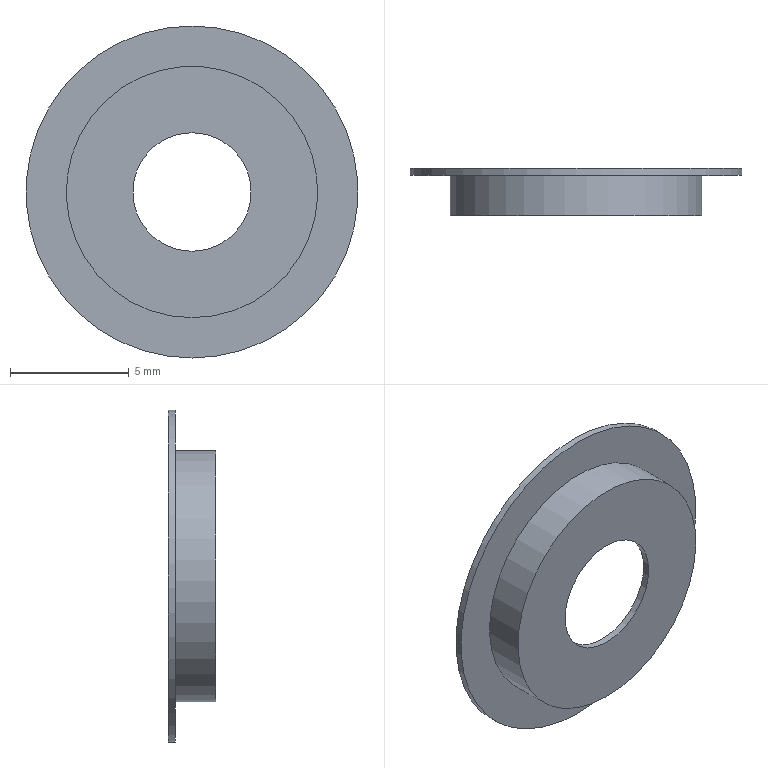Part | NX | features DATUM_CSYS 3, SKETCH 2, SWP104 1 | 1 solid | 8 faces | box 14 x 2 x 14 mm | volume 56.794 mm3 | cylinder 4 | plane 4 | commonest cylinder face diameters 5 x1 10 x1 10.6 x1 14 x1
STEP:
#1=CARTESIAN_POINT('',(0.,0.,-5.));
#2=VERTEX_POINT('',#1);
#3=CARTESIAN_POINT('',(0.,0.,0.));
#4=DIRECTION('',(0.,-1.,0.));
#5=DIRECTION('',(0.,0.,-1.));
#6=AXIS2_PLACEMENT_3D('',#3,#4,#5);
#7=CIRCLE('',#6,5.);
#8=EDGE_CURVE('',#2,#2,#7,.T.);
#9=ORIENTED_EDGE('',*,*,#8,.T.);
#10=EDGE_LOOP('',(#9));
#11=FACE_BOUND('',#10,.T.);
#12=CARTESIAN_POINT('',(0.,1.7,-5.));
#13=VERTEX_POINT('',#12);
#14=CARTESIAN_POINT('',(0.,1.7,0.));
#15=DIRECTION('',(0.,-1.,0.));
#16=DIRECTION('',(0.,0.,-1.));
#17=AXIS2_PLACEMENT_3D('',#14,#15,#16);
#18=CIRCLE('',#17,5.);
#19=EDGE_CURVE('',#13,#13,#18,.T.);
#20=ORIENTED_EDGE('',*,*,#19,.F.);
#21=EDGE_LOOP('',(#20));
#22=FACE_BOUND('',#21,.T.);
#23=CARTESIAN_POINT('',(0.,0.,0.));
#24=DIRECTION('',(0.,-1.,0.));
#25=DIRECTION('',(0.,0.,-1.));
#26=AXIS2_PLACEMENT_3D('',#23,#24,#25);
#27=CYLINDRICAL_SURFACE('',#26,5.);
#28=ADVANCED_FACE('',(#11,#22),#27,.F.);
#29=CARTESIAN_POINT('',(0.,0.,-2.5));
#30=VERTEX_POINT('',#29);
#31=CARTESIAN_POINT('',(0.,0.,0.));
#32=DIRECTION('',(0.,-1.,0.));
#33=DIRECTION('',(0.,0.,-1.));
#34=AXIS2_PLACEMENT_3D('',#31,#32,#33);
#35=CIRCLE('',#34,2.5);
#36=EDGE_CURVE('',#30,#30,#35,.T.);
#37=ORIENTED_EDGE('',*,*,#36,.T.);
#38=EDGE_LOOP('',(#37));
#39=FACE_BOUND('',#38,.T.);
#40=ORIENTED_EDGE('',*,*,#8,.F.);
#41=EDGE_LOOP('',(#40));
#42=FACE_BOUND('',#41,.T.);
#43=CARTESIAN_POINT('',(0.,0.,5.));
#44=DIRECTION('',(0.,1.,0.));
#45=DIRECTION('',(0.,0.,1.));
#46=AXIS2_PLACEMENT_3D('',#43,#44,#45);
#47=PLANE('',#46);
#48=ADVANCED_FACE('',(#39,#42),#47,.T.);
#49=CARTESIAN_POINT('',(0.,-0.3,-2.5));
#50=VERTEX_POINT('',#49);
#51=CARTESIAN_POINT('',(0.,-0.3,0.));
#52=DIRECTION('',(0.,-1.,0.));
#53=DIRECTION('',(0.,0.,-1.));
#54=AXIS2_PLACEMENT_3D('',#51,#52,#53);
#55=CIRCLE('',#54,2.5);
#56=EDGE_CURVE('',#50,#50,#55,.T.);
#57=ORIENTED_EDGE('',*,*,#56,.T.);
#58=EDGE_LOOP('',(#57));
#59=FACE_BOUND('',#58,.T.);
#60=ORIENTED_EDGE('',*,*,#36,.F.);
#61=EDGE_LOOP('',(#60));
#62=FACE_BOUND('',#61,.T.);
#63=CARTESIAN_POINT('',(0.,0.,0.));
#64=DIRECTION('',(0.,-1.,0.));
#65=DIRECTION('',(0.,0.,-1.));
#66=AXIS2_PLACEMENT_3D('',#63,#64,#65);
#67=CYLINDRICAL_SURFACE('',#66,2.5);
#68=ADVANCED_FACE('',(#59,#62),#67,.F.);
#69=CARTESIAN_POINT('',(0.,-0.3,-5.3));
#70=VERTEX_POINT('',#69);
#71=CARTESIAN_POINT('',(0.,-0.3,0.));
#72=DIRECTION('',(0.,-1.,0.));
#73=DIRECTION('',(0.,0.,-1.));
#74=AXIS2_PLACEMENT_3D('',#71,#72,#73);
#75=CIRCLE('',#74,5.3);
#76=EDGE_CURVE('',#70,#70,#75,.T.);
#77=ORIENTED_EDGE('',*,*,#76,.T.);
#78=EDGE_LOOP('',(#77));
#79=FACE_BOUND('',#78,.T.);
#80=ORIENTED_EDGE('',*,*,#56,.F.);
#81=EDGE_LOOP('',(#80));
#82=FACE_BOUND('',#81,.T.);
#83=CARTESIAN_POINT('',(0.,-0.3,2.5));
#84=DIRECTION('',(0.,-1.,0.));
#85=DIRECTION('',(0.,0.,-1.));
#86=AXIS2_PLACEMENT_3D('',#83,#84,#85);
#87=PLANE('',#86);
#88=ADVANCED_FACE('',(#79,#82),#87,.T.);
#89=CARTESIAN_POINT('',(0.,1.4,-5.3));
#90=VERTEX_POINT('',#89);
#91=CARTESIAN_POINT('',(0.,1.4,0.));
#92=DIRECTION('',(0.,-1.,0.));
#93=DIRECTION('',(0.,0.,-1.));
#94=AXIS2_PLACEMENT_3D('',#91,#92,#93);
#95=CIRCLE('',#94,5.3);
#96=EDGE_CURVE('',#90,#90,#95,.T.);
#97=ORIENTED_EDGE('',*,*,#96,.T.);
#98=EDGE_LOOP('',(#97));
#99=FACE_BOUND('',#98,.T.);
#100=ORIENTED_EDGE('',*,*,#76,.F.);
#101=EDGE_LOOP('',(#100));
#102=FACE_BOUND('',#101,.T.);
#103=CARTESIAN_POINT('',(0.,0.,0.));
#104=DIRECTION('',(0.,-1.,0.));
#105=DIRECTION('',(0.,0.,-1.));
#106=AXIS2_PLACEMENT_3D('',#103,#104,#105);
#107=CYLINDRICAL_SURFACE('',#106,5.3);
#108=ADVANCED_FACE('',(#99,#102),#107,.T.);
#109=CARTESIAN_POINT('',(0.,1.4,-7.));
#110=VERTEX_POINT('',#109);
#111=CARTESIAN_POINT('',(0.,1.4,0.));
#112=DIRECTION('',(0.,-1.,0.));
#113=DIRECTION('',(0.,0.,-1.));
#114=AXIS2_PLACEMENT_3D('',#111,#112,#113);
#115=CIRCLE('',#114,7.);
#116=EDGE_CURVE('',#110,#110,#115,.T.);
#117=ORIENTED_EDGE('',*,*,#116,.T.);
#118=EDGE_LOOP('',(#117));
#119=FACE_BOUND('',#118,.T.);
#120=ORIENTED_EDGE('',*,*,#96,.F.);
#121=EDGE_LOOP('',(#120));
#122=FACE_BOUND('',#121,.T.);
#123=CARTESIAN_POINT('',(0.,1.4,5.3));
#124=DIRECTION('',(0.,-1.,0.));
#125=DIRECTION('',(0.,0.,-1.));
#126=AXIS2_PLACEMENT_3D('',#123,#124,#125);
#127=PLANE('',#126);
#128=ADVANCED_FACE('',(#119,#122),#127,.T.);
#129=CARTESIAN_POINT('',(0.,1.7,-7.));
#130=VERTEX_POINT('',#129);
#131=CARTESIAN_POINT('',(0.,1.7,0.));
#132=DIRECTION('',(0.,-1.,0.));
#133=DIRECTION('',(0.,0.,-1.));
#134=AXIS2_PLACEMENT_3D('',#131,#132,#133);
#135=CIRCLE('',#134,7.);
#136=EDGE_CURVE('',#130,#130,#135,.T.);
#137=ORIENTED_EDGE('',*,*,#136,.T.);
#138=EDGE_LOOP('',(#137));
#139=FACE_BOUND('',#138,.T.);
#140=ORIENTED_EDGE('',*,*,#116,.F.);
#141=EDGE_LOOP('',(#140));
#142=FACE_BOUND('',#141,.T.);
#143=CARTESIAN_POINT('',(0.,0.,0.));
#144=DIRECTION('',(0.,-1.,0.));
#145=DIRECTION('',(0.,0.,-1.));
#146=AXIS2_PLACEMENT_3D('',#143,#144,#145);
#147=CYLINDRICAL_SURFACE('',#146,7.);
#148=ADVANCED_FACE('',(#139,#142),#147,.T.);
#149=ORIENTED_EDGE('',*,*,#19,.T.);
#150=EDGE_LOOP('',(#149));
#151=FACE_BOUND('',#150,.T.);
#152=ORIENTED_EDGE('',*,*,#136,.F.);
#153=EDGE_LOOP('',(#152));
#154=FACE_BOUND('',#153,.T.);
#155=CARTESIAN_POINT('',(0.,1.7,7.));
#156=DIRECTION('',(0.,1.,0.));
#157=DIRECTION('',(0.,0.,1.));
#158=AXIS2_PLACEMENT_3D('',#155,#156,#157);
#159=PLANE('',#158);
#160=ADVANCED_FACE('',(#151,#154),#159,.T.);
#161=CLOSED_SHELL('',(#28,#48,#68,#88,#108,#128,#148,#160));
#162=MANIFOLD_SOLID_BREP('',#161);
#163=(LENGTH_UNIT()NAMED_UNIT(*)SI_UNIT(.MILLI.,.METRE.));
#164=UNCERTAINTY_MEASURE_WITH_UNIT(LENGTH_MEASURE(0.00001),#163,'','');
#165=(NAMED_UNIT(*)PLANE_ANGLE_UNIT()SI_UNIT($,.RADIAN.));
#166=(NAMED_UNIT(*)SI_UNIT($,.STERADIAN.)SOLID_ANGLE_UNIT());
#167=(GEOMETRIC_REPRESENTATION_CONTEXT(3)GLOBAL_UNCERTAINTY_ASSIGNED_CONTEXT((#164))GLOBAL_UNIT_ASSIGNED_CONTEXT((#163,#165,#166))REPRESENTATION_CONTEXT('',''));
#168=ADVANCED_BREP_SHAPE_REPRESENTATION('',(#162),#167);